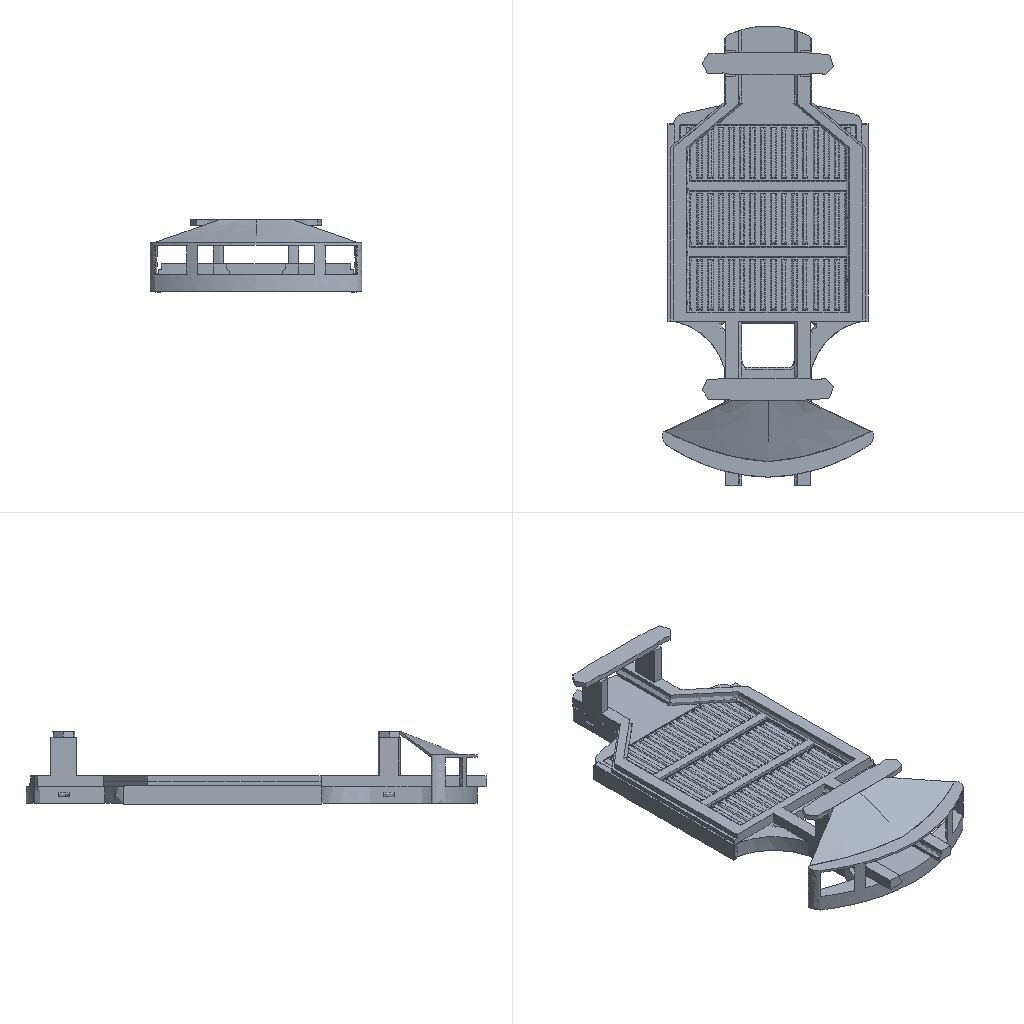Simulation study | ansys workbench
Ansys APDL input file, long lists of numbers shortened:
/batch
/config,noeldb,1     ! force off writing results to database
*get,_wallstrt,active,,time,wall
! ANSYS input file written by Workbench version 2022 R1
! File used for geometry attach: F:\ansys（分析文件汇总)\底盘有限元分析\ansys\dipan.STEP
/title,wbnew--____ (D5)
! ****** Begin Custom Load Command Snippet ******
/COM, ACT Extensions:
/COM,     LSDYNA, 2021.1
/COM,
! ****** End   Custom Load Command Snippet ******
*DIM,_wb_ProjectScratch_dir,string,248
_wb_ProjectScratch_dir(1) = 'C:\Users\Administrator\AppData\Local\Temp\WB_Administrator_26060_2\_ProjectScratch\ScrF2AA\'
*DIM,_wb_SolverFiles_dir,string,248
_wb_SolverFiles_dir(1) = 'C:\Users\Administrator\AppData\Local\Temp\WB_Administrator_26060_2\wbnew_files\dp0\SYS-2\MECH\'
*DIM,_wb_userfiles_dir,string,248
_wb_userfiles_dir(1) = 'C:\Users\Administrator\AppData\Local\Temp\WB_Administrator_26060_2\wbnew_files\user_files\'
/com,--- Data in consistent NMM units. See Solving Units in the help system for more information.
/units,MPA
/nopr
/wb,file,start              !  signify a WB generated input file
/prep7
! Turn off shape checking because checks already performed inside WB mesher.
! See help system for more information.
SHPP,OFF,,NOWARN
/nolist
etcon,set             ! allow ANSYS to choose best KEYOP's for 180x elements, resets any applicable keyopt to MAPDL defaults
/com,*********** Nodes for the whole assembly ***********
nblock,3,,302792
(1i9,3e20.9e3)
        1    -4.943372315E+02    -3.667689240E+02     3.655805537E+02
! (275265 more lines like these left out)
-1
/wb,elem,start            !  set before creation of elements
/com,*********** Elements for Body 1 "dipan-FreeParts|NONE" ***********
et,1,187
eblock,19,solid,,173485
(19i9)
        1        1        1        1        0        0        0        0       10        0       19    13623    39379    40222    40211   140088   275016   140091   140090
! (346969 more lines like these left out)
-1
/com,*********** Elements for Body 2 "dipan-FreeParts|NONE[2]" ***********
et,2,186
keyo,2,2,1          ! set full integration on SOLID186
eblock,19,solid,,9
(19i9)
        2        2        2        2        0        0        0        0       20        0       10      100      117      120      121      101      115      116      112
! (17 more lines like these left out)
-1
/com,*********** Elements for Body 3 "dipan-FreeParts|NONE[3]" ***********
et,3,186
keyo,3,2,1          ! set full integration on SOLID186
eblock,19,solid,,9
(19i9)
        3        3        3        3        0        0        0        0       20        0        1        4       21       24       25        5       19       20       16
! (17 more lines like these left out)
-1
/wb,elem,end               !  done creating elements
/com,*********** Send User Defined Coordinate System(s) ***********
csys,0
toffst,273.15,  ! Temperature offset from absolute zero
/com,*********** Set Reference Temperature ***********
tref,22.
/wb,mat,start              !  starting to send materials
/com,*********** Send Materials ***********
Temperature = 'TEMP' ! Temperature
MP,DENS,1,7.85e-09,	! tonne mm^-3
MP,ALPX,1,1.2e-05,	! C^-1
MP,C,1,434000000,	! mm^2 s^-2 C^-1
MP,KXX,1,60.5,	! tonne mm s^-3 C^-1
MP,RSVX,1,0.00017,	! ohm mm
MP,EX,1,200000,	! tonne s^-2 mm^-1
MP,NUXY,1,0.3,
MP,MURX,1,10000,
Temperature = 'TEMP' ! Temperature
MP,DENS,2,7.85e-09,	! tonne mm^-3
MP,ALPX,2,1.2e-05,	! C^-1
MP,C,2,434000000,	! mm^2 s^-2 C^-1
MP,KXX,2,60.5,	! tonne mm s^-3 C^-1
MP,RSVX,2,0.00017,	! ohm mm
MP,EX,2,200000,	! tonne s^-2 mm^-1
MP,NUXY,2,0.3,
MP,MURX,2,10000,
Temperature = 'TEMP' ! Temperature
MP,DENS,3,7.85e-09,	! tonne mm^-3
MP,ALPX,3,1.2e-05,	! C^-1
MP,C,3,434000000,	! mm^2 s^-2 C^-1
MP,KXX,3,60.5,	! tonne mm s^-3 C^-1
MP,RSVX,3,0.00017,	! ohm mm
MP,EX,3,200000,	! tonne s^-2 mm^-1
MP,NUXY,3,0.3,
MP,MURX,3,10000,
/wb,mat,end                !  done sending materials
!************************* Model Summary ********************
!dipan-FreeParts|NONE,	结构钢,	matid,	1
!dipan-FreeParts|NONE[2],	结构钢,	matid,	2
!dipan-FreeParts|NONE[3],	结构钢,	matid,	3
!************************* End Model Summary ********************
! get the diagonal of the bounding box. Needed later for other things
*get,_xmin,node,,mnloc,x
*get,_ymin,node,,mnloc,y
*get,_zmin,node,,mnloc,z
*get,_xmax,node,,mxloc,x
*get,_ymax,node,,mxloc,y
*get,_zmax,node,,mxloc,z
_ASMDIAG=(_xmax-_xmin)*(_xmax-_xmin)+(_ymax-_ymin)*(_ymax-_ymin)+(_zmax-_zmin)*(_zmax-_zmin)
_ASMDIAG=SQRT(_ASMDIAG)
/wb,contact,start          !  starting to send contact
/com,*********** Create Contact "接触区域 3" ***********
/com,            Real Constant Set For Above Contact Is 5 & 4
*set,tid,5
*set,cid,4
r,tid
r,cid
et,tid,170
et,cid,174
eblock,10,,,3
(15i9)
   216164        5        5        5        0      126      125      108      107      190      165      162      163
   216165        5        5        5        0      125      124      109      108      189      167      164      165
   216166        5        5        5        0      124      119      113      109      184      175      166      167
-1
eblock,10,,,3
(15i9)
   216167        4        4        4        0      126      125      108      107      190      165      162      163
   216168        4        4        4        0      125      124      109      108      189      167      164      165
   216169        4        4        4        0      124      119      113      109      184      175      166      167
-1
eblock,10,,,3
(15i9)
   216170        4        5        4        0       14       15       26       27       72       75       91       73
   216171        4        5        4        0       15       16       25       26       74       77       90       75
   216172        4        5        4        0       16       20       24       25       76       84       89       77
-1
eblock,10,,,3
(15i9)
   216173        5        4        5        0       14       15       26       27       72       75       91       73
   216174        5        4        5        0       15       16       25       26       74       77       90       75
   216175        5        4        5        0       16       20       24       25       76       84       89       77
-1
keyo,cid,8,2               ! auto create asymmetric contact (from Program Controlled setting)
keyo,cid,10,0              ! adjust contact stiffness each NR iteration (from Program Controlled setting)
keyo,cid,12,5              ! bonded always
keyo,cid,18,1              ! small sliding turned on by application
keyo,cid,2,0               ! augmented Lagrange (from Program Controlled setting)
keyo,cid,4,0               ! on Gauss point (from Program Controlled setting)
keyo,cid,9,1               ! ignore initial gaps/penetration
keyo,cid,7,0               ! No Prediction
rmod,tid,3,10.      ! FKN
rmod,tid,5,0.       ! ICONT
rmod,tid,6,0.       ! PINB
rmod,tid,10,0.      ! CNOF
rmod,tid,12,0.      ! FKT
rmod,tid,36,47      ! WB DSID
rmod,cid,3,10.      ! FKN
rmod,cid,5,0.       ! ICONT
rmod,cid,6,0.       ! PINB
rmod,cid,10,0.      ! CNOF
rmod,cid,12,0.      ! FKT
rmod,cid,36,47      ! WB DSID
nsel,all
esel,all
/wb,contact,end            !  done creating contacts
/golist
/wb,load,start             !  starting to send loads
/com,*********** Fixed Supports ***********
CMBLOCK,_FIXEDSU,NODE,      648
(8i10)
         5         6         7         8         9        10        11        12
! (80 more lines like these left out)
cmsel,s,_FIXEDSU
d,all,all
nsel,all
/com,*********** Define Force Using Surface Effect Elements ***********
local,12,0,0.,0.,0.,0.,0.,0.
csys,0
et,6,154
eblock,10,,,289
(15i9)
   216176        6        6        6       12    20132    20151    20156    20156   171814   171938    20156   171815
! (288 more lines like these left out)
-1
esel,s,type,,6
keyop,6,2,1                ! Apply load in local coordinate system
keyop,6,7,1                ! Use original area so load is constant in large deformation
esel,all
/gst,on,on
fini
*get,_numnode,node,0,count
*get,_numelem,elem,0,count
*get, _MAXELEMNUM, elem, 0, NUM, MAX
*get, _MAXNODENUM, node, 0, NUM, MAX
*get, _MAXELEMTYPE, etyp, 0, NUM, MAX
*get, _MAXREALCONST, real, 0, NUM, MAX
/go
/wb,load,end               !  done creating loads
/com,--- Number of total nodes = %_numnode%
/com,--- Number of contact elements = 301
/com,--- Number of spring elements = 0
/com,--- Number of bearing elements = 0
/com,--- Number of solid elements = 173503
/com,--- Number of condensed parts = 0
/com,--- Number of total elements = %_numelem%
*get,_wallbsol,active,,time,wall
/com,****************************************************************************
/com,*************************    SOLUTION       ********************************
/com,****************************************************************************
/solu
antype,0                   ! static analysis
_thickRatio=0.333   ! Ratio of thick parts in the model
eqsl,sparse,,,,,1
cntr,print,1               ! print out contact info and also make no initial contact an error
dmpoption,emat,no             ! Don't combine emat file for DANSYS
dmpoption,esav,no             ! Don't combine esav file for DANSYS
nldiag,cont,iter           ! print out contact info each equilibrium iteration
rescontrol,,none                 ! Do not keep any restart files
/com,****************************************************
/com,******************* SOLVE FOR LS 1 OF 1 ****************
esel,s,type,,6
nsle
sfe,all,1,pres,1,0.
sfe,all,2,pres,1,4.674
sfe,all,3,pres,1,0.
nsel,all
esel,all
/nopr
/gopr
nsub,1,1,1
time,1.
outres,erase
outres,all,none
outres,nsol,all,
outres,rsol,all
outres,eangl,all
outres,etmp,all
outres,veng,all
outres,strs,all,
outres,epel,all,
outres,eppl,all,
outres,cont,all,
! *********** WB SOLVE COMMAND ***********
! check interactive state
*get,ANSINTER_,active,,int
*if,ANSINTER_,ne,0,then
/eof
*endif
solve
/com *************** Write FE CONNECTORS *********
CEWRITE,file,ce,,INTE
/com,****************************************************
/com,*************** FINISHED SOLVE FOR LS 1 *************
*get,_wallasol,active,,time,wall
/nopr
*get,_numnode,node,0,count
*get,_numelem,elem,0,count
*get, _MAXELEMNUM, elem, 0, NUM, MAX
*get, _MAXNODENUM, node, 0, NUM, MAX,,,INTERNAL
*get, _MAXELEMTYPE, etyp, 0, NUM, MAX
*get, _MAXREALCONST, real, 0, NUM, MAX
/gopr
/post1
xmlo,ENCODING,ISO-8859-1
xmlo,parm
/xml,parm,xml
fini
/gopr
*get,_walldone,active,,time,wall
_preptime=(_wallbsol-_wallstrt)*3600
_solvtime=(_wallasol-_wallbsol)*3600
_posttime=(_walldone-_wallasol)*3600
_totaltim=(_walldone-_wallstrt)*3600
*get,_dlbratio,active,0,solu,dlbr
*get,_combtime,active,0,solu,comb
*get,_ssmode,active,0,solu,ssmm
*get,_ndofs,active,0,solu,ndof
*get,_sol_end_time,active,0,set,time
*if,_sol_end_time,eq,1.,then
/fclean				!clean distributed files
*endif
/com,--- Total number of nodes = %_numnode%
/com,--- Total number of elements = %_numelem%
/com,--- Element load balance ratio = %_dlbratio%
/com,--- Time to combine distributed files = %_combtime%
/com,--- Sparse memory mode = %_ssmode%
/com,--- Number of DOF = %_ndofs%
/wb,file,end               ! done with WB generated input